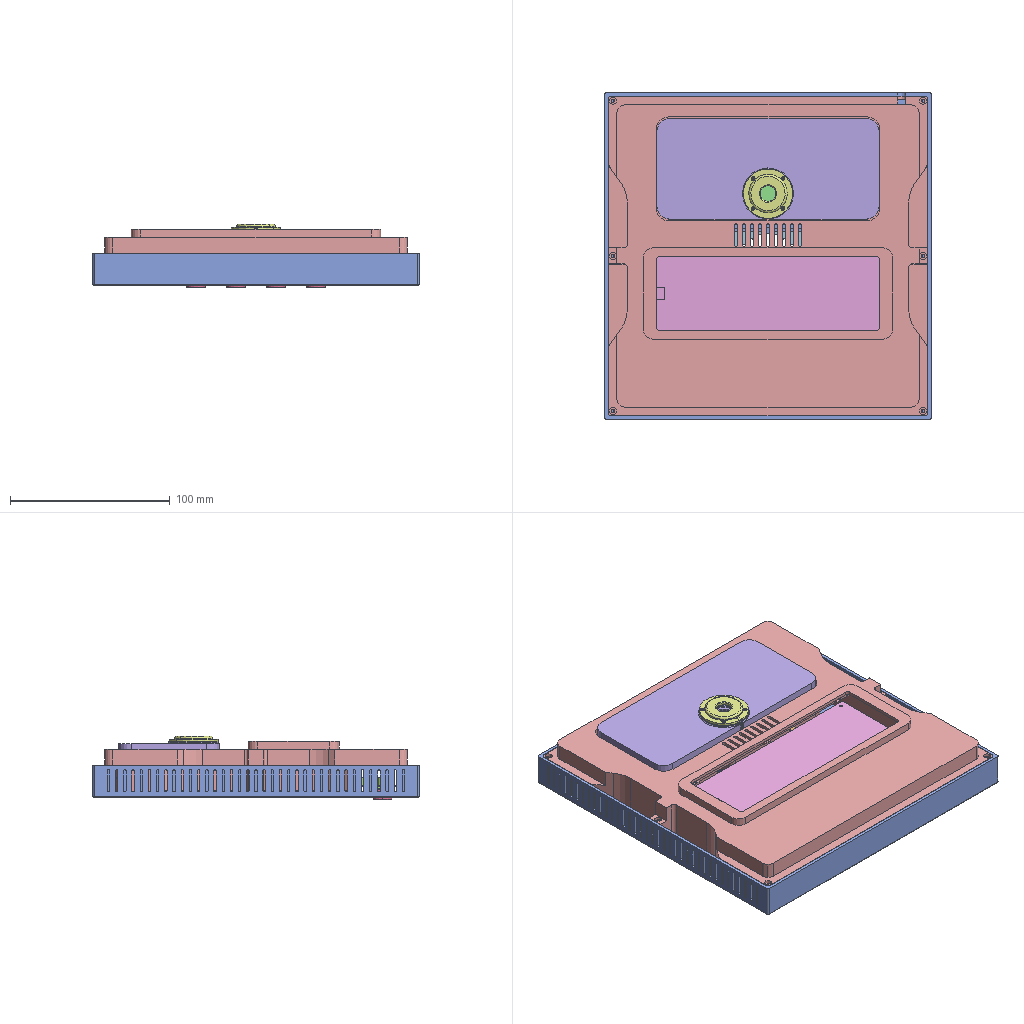Assembly | SolidWorks | 12 different items | 12 placed | box 204 x 204 x 40 mm
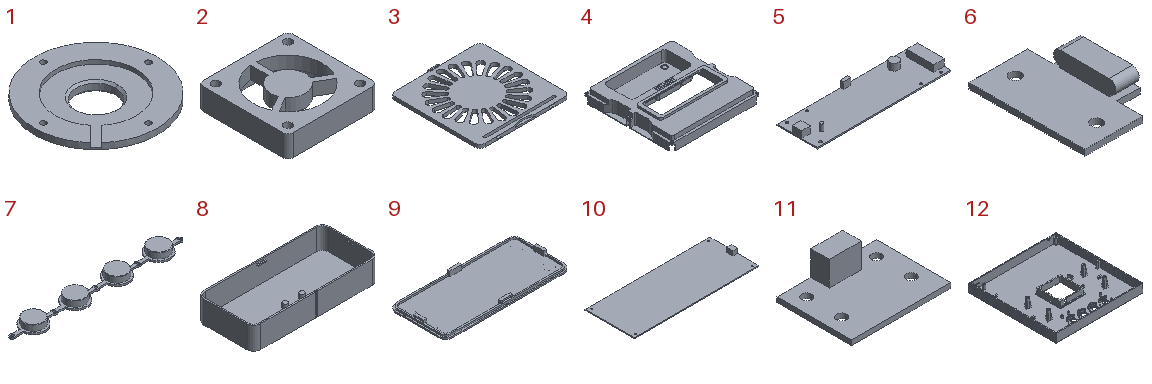Parts list (item | quantity | size | volume | features):
1 | x1 | 31 x 31 x 3.5 mm | 1459 mm3 | features ICE 5, Chamfer 1, Extrusion 1, Fillet 1
2 | x1 | 50 x 50 x 12 mm | 16391 mm3 | features ICE 2, Extrusion 1
3 | x1 | 52.5 x 54.75 x 2.2 mm | 3927 mm3 | features ICE 4, Extrusion 1, MirrorPattern 1
4 | x1 | 199.7 x 199.7 x 33 mm | 138298 mm3 | features ICE 31, Fillet 3, Chamfer 1, Extrusion 1, LPattern 1, MirrorPattern 1, Shell 1
5 | x1 | 100 x 30 x 8 mm | 4377 mm3 | features ICE 4, Extrusion 1
6 | x1 | 14 x 20 x 3.696 mm | 327.493 mm3 | features ICE 4, Extrusion 1
7 | x1 | 103 x 14 x 6.5 mm | 2380 mm3 | features Chamfer 2, ICE 2, Extrusion 1
8 | x1 | 139 x 63 x 26.2 mm | 27399 mm3 | features ICE 11, Fillet 4, Chamfer 2, MirrorPattern 2, Extrusion 1, Shell 1
9 | x1 | 139 x 63 x 8 mm | 14541 mm3 | features ICE 7, MirrorPattern 2, Extrusion 1
10 | x1 | 140 x 55 x 6 mm | 7876 mm3 | features Extrusion 1, ICE 1
11 | x1 | 20 x 15 x 6 mm | 407.762 mm3 | features Extrusion 1, ICE 1
12 | x1 | 204 x 204 x 24 mm | 116811 mm3 | features ICE 29, Fillet 5, Chamfer 3, Extrusion 1, MirrorPattern 1, Shell 1
Mates (type | each side: item.copy, entity, surface, feature):
Parallel | 4.1 face plane Boss-Extrude2 | 12.1 face plane Boss-Extrude1
Coincident | 4.1 face plane Boss-Extrude1 | 12.1 face plane Shell1
DistanceDim | 5.1 face plane Boss-Extrude1 | 12.1 face plane Boss-Extrude1
DistanceDim | 10.1 face plane Boss-Extrude1 | 4.1 face plane Shell1
DistanceDim | 2.1 face plane Boss-Extrude1 | 12.1 face plane Cut-Extrude1 | 2 times
DistanceDim | 6.1 face plane Boss-Extrude1 | 4.1 face plane Boss-Extrude1
DistanceDim | 2.1 face plane Boss-Extrude1 | 12.1 face plane Cut-Extrude4
DistanceDim | 4.1 face plane Shell1 | 10.1 face plane Boss-Extrude1
Coincident | 12.1 face plane Boss-Extrude5 | 5.1 face plane Boss-Extrude1
DistanceDim | 11.1 face plane Boss-Extrude1 | 12.1 face plane Shell1
Coincident | 8.1 face plane Boss-Extrude1 | 9.1 face plane Boss-Extrude1 | 4 times
DistanceDim | 8.1 face plane Boss-Extrude1 | 4.1 face plane Cut-Extrude3 | 2 times
Concentric | 12.1 face cylinder Cut-Extrude1 | 7.1 face cylinder Boss-Extrude2 | 2 times
Coincident | 12.1 face plane Shell1 | 7.1 face plane Boss-Extrude1
DistanceDim | 3.1 face plane Boss-Extrude1 | 12.1 face plane Cut-Extrude4 | 2 times
Coincident | 12.1 face plane Boss-Extrude1 | 3.1 face plane Boss-Extrude1
Coincident | 4.1 face plane Boss-Extrude5 | 9.1 face plane Boss-Extrude2
Concentric | 8.1 face cylinder Cut-Extrude4 | 1.1 face cylinder Boss-Extrude2
Coincident | 1.1 face plane Boss-Extrude2 | 8.1 face plane Boss-Extrude7
Concentric | 8.1 face cylinder Cut-Extrude5 | 1.1 face cylinder Cut-Extrude2
DistanceDim | 4.1 face plane Cut-Extrude11 | 12.1 face plane Shell1 | 2 times
Concentric | 12.1 face cylinder Boss-Extrude8 | 11.1 face cylinder Boss-Extrude1 | 2 times
DistanceDim | 10.1 vertex | 4.1 face plane Boss-Extrude4